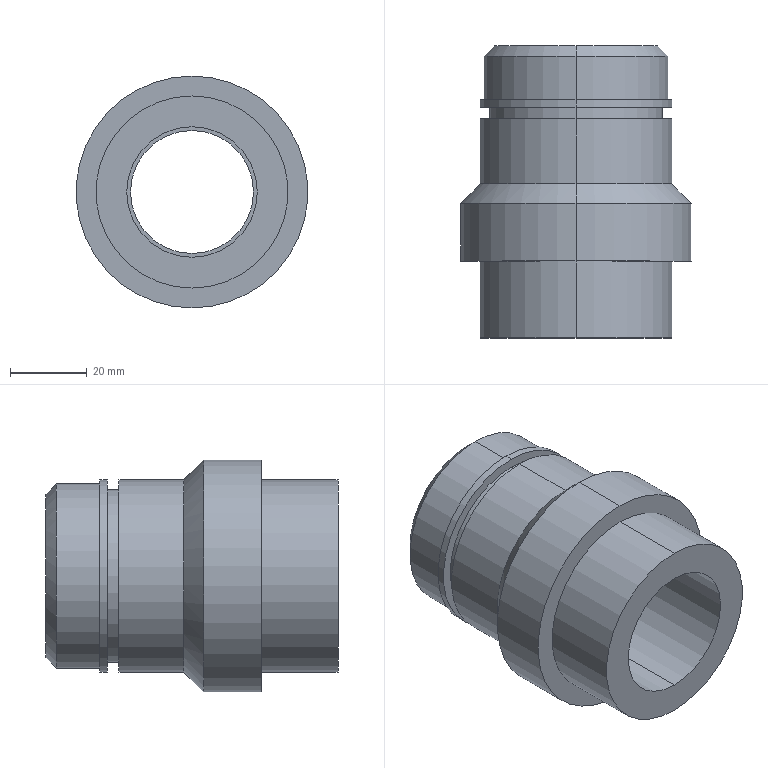Part | SolidWorks | features ICE 7, HoleWzd 2, Chamfer 1, Extrusion 1, StudWizard 1 | 1 solid | 27 faces | box 60.3 x 76 x 60.3 mm | volume 93894 mm3 | cylinder 16 | plane 7 | cone 4 | commonest cylinder face diameters 50 x6 32 x2 34 x2 45 x2 48 x2 60.3 x2
STEP:
#1=CARTESIAN_POINT('',(0.,58.,-16.));
#2=VERTEX_POINT('',#1);
#3=CARTESIAN_POINT('',(0.,58.,16.));
#4=VERTEX_POINT('',#3);
#5=CARTESIAN_POINT('',(0.,58.,0.));
#6=DIRECTION('',(0.,1.,0.));
#7=DIRECTION('',(0.,0.,1.));
#8=AXIS2_PLACEMENT_3D('',#5,#6,#7);
#9=CIRCLE('',#8,16.);
#10=EDGE_CURVE('',#2,#4,#9,.T.);
#11=ORIENTED_EDGE('',*,*,#10,.F.);
#12=CARTESIAN_POINT('',(0.,76.,-16.));
#13=VERTEX_POINT('',#12);
#14=CARTESIAN_POINT('',(0.,76.,-16.));
#15=DIRECTION('',(0.,1.,0.));
#16=VECTOR('',#15,1000.);
#17=LINE('',#14,#16);
#18=EDGE_CURVE('',#2,#13,#17,.T.);
#19=ORIENTED_EDGE('',*,*,#18,.T.);
#20=CARTESIAN_POINT('',(0.,76.,16.));
#21=VERTEX_POINT('',#20);
#22=CARTESIAN_POINT('',(0.,76.,0.));
#23=DIRECTION('',(0.,1.,0.));
#24=DIRECTION('',(0.,0.,1.));
#25=AXIS2_PLACEMENT_3D('',#22,#23,#24);
#26=CIRCLE('',#25,16.);
#27=EDGE_CURVE('',#13,#21,#26,.T.);
#28=ORIENTED_EDGE('',*,*,#27,.T.);
#29=CARTESIAN_POINT('',(0.,76.,16.));
#30=DIRECTION('',(0.,1.,0.));
#31=VECTOR('',#30,1000.);
#32=LINE('',#29,#31);
#33=EDGE_CURVE('',#4,#21,#32,.T.);
#34=ORIENTED_EDGE('',*,*,#33,.F.);
#35=EDGE_LOOP('',(#11,#19,#28,#34));
#36=FACE_OUTER_BOUND('',#35,.T.);
#37=CARTESIAN_POINT('',(0.,76.,0.));
#38=DIRECTION('',(0.,1.,0.));
#39=DIRECTION('',(0.,0.,1.));
#40=AXIS2_PLACEMENT_3D('',#37,#38,#39);
#41=CYLINDRICAL_SURFACE('',#40,16.);
#42=ADVANCED_FACE('',(#36),#41,.F.);
#43=CARTESIAN_POINT('',(0.,58.,17.));
#44=VERTEX_POINT('',#43);
#45=CARTESIAN_POINT('',(0.,58.,-17.));
#46=VERTEX_POINT('',#45);
#47=CARTESIAN_POINT('',(0.,58.,0.));
#48=DIRECTION('',(0.,-1.,0.));
#49=DIRECTION('',(0.,0.,1.));
#50=AXIS2_PLACEMENT_3D('',#47,#48,#49);
#51=CIRCLE('',#50,17.);
#52=EDGE_CURVE('',#44,#46,#51,.T.);
#53=ORIENTED_EDGE('',*,*,#52,.F.);
#54=CARTESIAN_POINT('',(0.,0.,17.));
#55=VERTEX_POINT('',#54);
#56=CARTESIAN_POINT('',(0.,0.,17.));
#57=DIRECTION('',(0.,-1.,0.));
#58=VECTOR('',#57,1000.);
#59=LINE('',#56,#58);
#60=EDGE_CURVE('',#44,#55,#59,.T.);
#61=ORIENTED_EDGE('',*,*,#60,.T.);
#62=CARTESIAN_POINT('',(0.,0.,-17.));
#63=VERTEX_POINT('',#62);
#64=CARTESIAN_POINT('',(0.,0.,0.));
#65=DIRECTION('',(0.,-1.,0.));
#66=DIRECTION('',(0.,0.,-1.));
#67=AXIS2_PLACEMENT_3D('',#64,#65,#66);
#68=CIRCLE('',#67,17.);
#69=EDGE_CURVE('',#55,#63,#68,.T.);
#70=ORIENTED_EDGE('',*,*,#69,.T.);
#71=CARTESIAN_POINT('',(0.,0.,-17.));
#72=DIRECTION('',(0.,-1.,0.));
#73=VECTOR('',#72,1000.);
#74=LINE('',#71,#73);
#75=EDGE_CURVE('',#46,#63,#74,.T.);
#76=ORIENTED_EDGE('',*,*,#75,.F.);
#77=EDGE_LOOP('',(#53,#61,#70,#76));
#78=FACE_OUTER_BOUND('',#77,.T.);
#79=CARTESIAN_POINT('',(0.,0.,0.));
#80=DIRECTION('',(0.,-1.,0.));
#81=DIRECTION('',(0.,0.,-1.));
#82=AXIS2_PLACEMENT_3D('',#79,#80,#81);
#83=CYLINDRICAL_SURFACE('',#82,17.);
#84=ADVANCED_FACE('',(#78),#83,.F.);
#85=CARTESIAN_POINT('',(0.,40.15,25.));
#86=VERTEX_POINT('',#85);
#87=CARTESIAN_POINT('',(0.,40.15,-25.));
#88=VERTEX_POINT('',#87);
#89=CARTESIAN_POINT('',(0.,40.15,0.));
#90=DIRECTION('',(0.,1.,0.));
#91=DIRECTION('',(0.,0.,-1.));
#92=AXIS2_PLACEMENT_3D('',#89,#90,#91);
#93=CIRCLE('',#92,25.);
#94=EDGE_CURVE('',#86,#88,#93,.T.);
#95=ORIENTED_EDGE('',*,*,#94,.F.);
#96=CARTESIAN_POINT('',(0.,35.,30.15));
#97=VERTEX_POINT('',#96);
#98=CARTESIAN_POINT('',(0.,35.,30.15));
#99=DIRECTION('',(0.,-0.7071,0.7071));
#100=VECTOR('',#99,1000.);
#101=LINE('',#98,#100);
#102=EDGE_CURVE('',#86,#97,#101,.T.);
#103=ORIENTED_EDGE('',*,*,#102,.T.);
#104=CARTESIAN_POINT('',(0.,35.,-30.15));
#105=VERTEX_POINT('',#104);
#106=CARTESIAN_POINT('',(0.,35.,0.));
#107=DIRECTION('',(0.,-1.,0.));
#108=DIRECTION('',(0.,0.,-1.));
#109=AXIS2_PLACEMENT_3D('',#106,#107,#108);
#110=CIRCLE('',#109,30.15);
#111=EDGE_CURVE('',#105,#97,#110,.T.);
#112=ORIENTED_EDGE('',*,*,#111,.F.);
#113=CARTESIAN_POINT('',(0.,35.,-30.15));
#114=DIRECTION('',(0.,-0.7071,-0.7071));
#115=VECTOR('',#114,1000.);
#116=LINE('',#113,#115);
#117=EDGE_CURVE('',#88,#105,#116,.T.);
#118=ORIENTED_EDGE('',*,*,#117,.F.);
#119=EDGE_LOOP('',(#95,#103,#112,#118));
#120=FACE_OUTER_BOUND('',#119,.T.);
#121=CARTESIAN_POINT('',(0.,35.,0.));
#122=DIRECTION('',(0.,-1.,0.));
#123=DIRECTION('',(0.,0.,-1.));
#124=AXIS2_PLACEMENT_3D('',#121,#122,#123);
#125=CONICAL_SURFACE('',#124,30.15,0.7854);
#126=ADVANCED_FACE('',(#120),#125,.T.);
#127=CARTESIAN_POINT('',(0.,20.,-25.));
#128=VERTEX_POINT('',#127);
#129=CARTESIAN_POINT('',(0.,20.,25.));
#130=VERTEX_POINT('',#129);
#131=CARTESIAN_POINT('',(0.,20.,0.));
#132=DIRECTION('',(0.,-1.,0.));
#133=DIRECTION('',(0.,0.,-1.));
#134=AXIS2_PLACEMENT_3D('',#131,#132,#133);
#135=CIRCLE('',#134,25.);
#136=EDGE_CURVE('',#128,#130,#135,.T.);
#137=ORIENTED_EDGE('',*,*,#136,.T.);
#138=CARTESIAN_POINT('',(0.,0.,25.));
#139=VERTEX_POINT('',#138);
#140=CARTESIAN_POINT('',(0.,57.,25.));
#141=DIRECTION('',(0.,-1.,0.));
#142=VECTOR('',#141,1000.);
#143=LINE('',#140,#142);
#144=EDGE_CURVE('',#130,#139,#143,.T.);
#145=ORIENTED_EDGE('',*,*,#144,.T.);
#146=CARTESIAN_POINT('',(0.,0.,-25.));
#147=VERTEX_POINT('',#146);
#148=CARTESIAN_POINT('',(0.,0.,0.));
#149=DIRECTION('',(0.,1.,0.));
#150=DIRECTION('',(0.,0.,1.));
#151=AXIS2_PLACEMENT_3D('',#148,#149,#150);
#152=CIRCLE('',#151,25.);
#153=EDGE_CURVE('',#139,#147,#152,.T.);
#154=ORIENTED_EDGE('',*,*,#153,.T.);
#155=CARTESIAN_POINT('',(0.,57.,-25.));
#156=DIRECTION('',(0.,-1.,0.));
#157=VECTOR('',#156,1000.);
#158=LINE('',#155,#157);
#159=EDGE_CURVE('',#128,#147,#158,.T.);
#160=ORIENTED_EDGE('',*,*,#159,.F.);
#161=EDGE_LOOP('',(#137,#145,#154,#160));
#162=FACE_OUTER_BOUND('',#161,.T.);
#163=CARTESIAN_POINT('',(0.,57.,0.));
#164=DIRECTION('',(0.,-1.,0.));
#165=DIRECTION('',(0.,0.,-1.));
#166=AXIS2_PLACEMENT_3D('',#163,#164,#165);
#167=CYLINDRICAL_SURFACE('',#166,25.);
#168=ADVANCED_FACE('',(#162),#167,.T.);
#169=ORIENTED_EDGE('',*,*,#111,.T.);
#170=CARTESIAN_POINT('',(0.,20.,30.15));
#171=VERTEX_POINT('',#170);
#172=CARTESIAN_POINT('',(0.,35.,30.15));
#173=DIRECTION('',(0.,-1.,0.));
#174=VECTOR('',#173,1000.);
#175=LINE('',#172,#174);
#176=EDGE_CURVE('',#97,#171,#175,.T.);
#177=ORIENTED_EDGE('',*,*,#176,.T.);
#178=CARTESIAN_POINT('',(0.,20.,-30.15));
#179=VERTEX_POINT('',#178);
#180=CARTESIAN_POINT('',(0.,20.,0.));
#181=DIRECTION('',(0.,-1.,0.));
#182=DIRECTION('',(0.,0.,-1.));
#183=AXIS2_PLACEMENT_3D('',#180,#181,#182);
#184=CIRCLE('',#183,30.15);
#185=EDGE_CURVE('',#179,#171,#184,.T.);
#186=ORIENTED_EDGE('',*,*,#185,.F.);
#187=CARTESIAN_POINT('',(0.,35.,-30.15));
#188=DIRECTION('',(0.,-1.,0.));
#189=VECTOR('',#188,1000.);
#190=LINE('',#187,#189);
#191=EDGE_CURVE('',#105,#179,#190,.T.);
#192=ORIENTED_EDGE('',*,*,#191,.F.);
#193=EDGE_LOOP('',(#169,#177,#186,#192));
#194=FACE_OUTER_BOUND('',#193,.T.);
#195=CARTESIAN_POINT('',(0.,35.,0.));
#196=DIRECTION('',(0.,-1.,0.));
#197=DIRECTION('',(0.,0.,-1.));
#198=AXIS2_PLACEMENT_3D('',#195,#196,#197);
#199=CYLINDRICAL_SURFACE('',#198,30.15);
#200=ADVANCED_FACE('',(#194),#199,.T.);
#201=CARTESIAN_POINT('',(0.,76.,-21.294));
#202=VERTEX_POINT('',#201);
#203=CARTESIAN_POINT('',(0.,76.,21.294));
#204=VERTEX_POINT('',#203);
#205=CARTESIAN_POINT('',(0.,76.,0.));
#206=DIRECTION('',(0.,-1.,0.));
#207=DIRECTION('',(0.,0.,-1.));
#208=AXIS2_PLACEMENT_3D('',#205,#206,#207);
#209=CIRCLE('',#208,21.294);
#210=EDGE_CURVE('',#202,#204,#209,.T.);
#211=ORIENTED_EDGE('',*,*,#210,.T.);
#212=CARTESIAN_POINT('',(0.,73.294,24.));
#213=VERTEX_POINT('',#212);
#214=CARTESIAN_POINT('',(0.,76.,21.294));
#215=DIRECTION('',(0.,-0.7071,0.7071));
#216=VECTOR('',#215,1000.);
#217=LINE('',#214,#216);
#218=EDGE_CURVE('',#204,#213,#217,.T.);
#219=ORIENTED_EDGE('',*,*,#218,.T.);
#220=CARTESIAN_POINT('',(0.,73.294,-24.));
#221=VERTEX_POINT('',#220);
#222=CARTESIAN_POINT('',(0.,73.294,0.));
#223=DIRECTION('',(0.,-1.,0.));
#224=DIRECTION('',(0.,0.,-1.));
#225=AXIS2_PLACEMENT_3D('',#222,#223,#224);
#226=CIRCLE('',#225,24.);
#227=EDGE_CURVE('',#221,#213,#226,.T.);
#228=ORIENTED_EDGE('',*,*,#227,.F.);
#229=CARTESIAN_POINT('',(0.,76.,-21.294));
#230=DIRECTION('',(0.,-0.7071,-0.7071));
#231=VECTOR('',#230,1000.);
#232=LINE('',#229,#231);
#233=EDGE_CURVE('',#202,#221,#232,.T.);
#234=ORIENTED_EDGE('',*,*,#233,.F.);
#235=EDGE_LOOP('',(#211,#219,#228,#234));
#236=FACE_OUTER_BOUND('',#235,.T.);
#237=CARTESIAN_POINT('',(0.,76.,0.));
#238=DIRECTION('',(0.,-1.,0.));
#239=DIRECTION('',(0.,0.,-1.));
#240=AXIS2_PLACEMENT_3D('',#237,#238,#239);
#241=CONICAL_SURFACE('',#240,21.294,0.7854);
#242=ADVANCED_FACE('',(#236),#241,.T.);
#243=ORIENTED_EDGE('',*,*,#227,.T.);
#244=CARTESIAN_POINT('',(0.,62.,24.));
#245=VERTEX_POINT('',#244);
#246=CARTESIAN_POINT('',(0.,76.,24.));
#247=DIRECTION('',(0.,-1.,0.));
#248=VECTOR('',#247,1000.);
#249=LINE('',#246,#248);
#250=EDGE_CURVE('',#213,#245,#249,.T.);
#251=ORIENTED_EDGE('',*,*,#250,.T.);
#252=CARTESIAN_POINT('',(0.,62.,-24.));
#253=VERTEX_POINT('',#252);
#254=CARTESIAN_POINT('',(0.,62.,0.));
#255=DIRECTION('',(0.,-1.,0.));
#256=DIRECTION('',(0.,0.,-1.));
#257=AXIS2_PLACEMENT_3D('',#254,#255,#256);
#258=CIRCLE('',#257,24.);
#259=EDGE_CURVE('',#253,#245,#258,.T.);
#260=ORIENTED_EDGE('',*,*,#259,.F.);
#261=CARTESIAN_POINT('',(0.,76.,-24.));
#262=DIRECTION('',(0.,-1.,0.));
#263=VECTOR('',#262,1000.);
#264=LINE('',#261,#263);
#265=EDGE_CURVE('',#221,#253,#264,.T.);
#266=ORIENTED_EDGE('',*,*,#265,.F.);
#267=EDGE_LOOP('',(#243,#251,#260,#266));
#268=FACE_OUTER_BOUND('',#267,.T.);
#269=CARTESIAN_POINT('',(0.,76.,0.));
#270=DIRECTION('',(0.,-1.,0.));
#271=DIRECTION('',(0.,0.,-1.));
#272=AXIS2_PLACEMENT_3D('',#269,#270,#271);
#273=CYLINDRICAL_SURFACE('',#272,24.);
#274=ADVANCED_FACE('',(#268),#273,.T.);
#275=CARTESIAN_POINT('',(0.,62.,25.));
#276=VERTEX_POINT('',#275);
#277=CARTESIAN_POINT('',(0.,62.,-25.));
#278=VERTEX_POINT('',#277);
#279=CARTESIAN_POINT('',(0.,62.,0.));
#280=DIRECTION('',(0.,1.,0.));
#281=DIRECTION('',(0.,0.,1.));
#282=AXIS2_PLACEMENT_3D('',#279,#280,#281);
#283=CIRCLE('',#282,25.);
#284=EDGE_CURVE('',#276,#278,#283,.T.);
#285=ORIENTED_EDGE('',*,*,#284,.F.);
#286=CARTESIAN_POINT('',(0.,60.,25.));
#287=VERTEX_POINT('',#286);
#288=CARTESIAN_POINT('',(0.,62.,25.));
#289=DIRECTION('',(0.,-1.,0.));
#290=VECTOR('',#289,1000.);
#291=LINE('',#288,#290);
#292=EDGE_CURVE('',#276,#287,#291,.T.);
#293=ORIENTED_EDGE('',*,*,#292,.T.);
#294=CARTESIAN_POINT('',(0.,60.,-25.));
#295=VERTEX_POINT('',#294);
#296=CARTESIAN_POINT('',(0.,60.,0.));
#297=DIRECTION('',(0.,1.,0.));
#298=DIRECTION('',(0.,0.,1.));
#299=AXIS2_PLACEMENT_3D('',#296,#297,#298);
#300=CIRCLE('',#299,25.);
#301=EDGE_CURVE('',#287,#295,#300,.T.);
#302=ORIENTED_EDGE('',*,*,#301,.T.);
#303=CARTESIAN_POINT('',(0.,62.,-25.));
#304=DIRECTION('',(0.,-1.,0.));
#305=VECTOR('',#304,1000.);
#306=LINE('',#303,#305);
#307=EDGE_CURVE('',#278,#295,#306,.T.);
#308=ORIENTED_EDGE('',*,*,#307,.F.);
#309=EDGE_LOOP('',(#285,#293,#302,#308));
#310=FACE_OUTER_BOUND('',#309,.T.);
#311=CARTESIAN_POINT('',(0.,62.,0.));
#312=DIRECTION('',(0.,-1.,0.));
#313=DIRECTION('',(0.,0.,-1.));
#314=AXIS2_PLACEMENT_3D('',#311,#312,#313);
#315=CYLINDRICAL_SURFACE('',#314,25.);
#316=ADVANCED_FACE('',(#310),#315,.T.);
#317=CARTESIAN_POINT('',(0.,60.,22.5));
#318=VERTEX_POINT('',#317);
#319=CARTESIAN_POINT('',(0.,60.,-22.5));
#320=VERTEX_POINT('',#319);
#321=CARTESIAN_POINT('',(0.,60.,0.));
#322=DIRECTION('',(0.,1.,0.));
#323=DIRECTION('',(0.,0.,1.));
#324=AXIS2_PLACEMENT_3D('',#321,#322,#323);
#325=CIRCLE('',#324,22.5);
#326=EDGE_CURVE('',#318,#320,#325,.T.);
#327=ORIENTED_EDGE('',*,*,#326,.F.);
#328=CARTESIAN_POINT('',(0.,57.,22.5));
#329=VERTEX_POINT('',#328);
#330=CARTESIAN_POINT('',(0.,60.,22.5));
#331=DIRECTION('',(0.,-1.,0.));
#332=VECTOR('',#331,1000.);
#333=LINE('',#330,#332);
#334=EDGE_CURVE('',#318,#329,#333,.T.);
#335=ORIENTED_EDGE('',*,*,#334,.T.);
#336=CARTESIAN_POINT('',(0.,57.,-22.5));
#337=VERTEX_POINT('',#336);
#338=CARTESIAN_POINT('',(0.,57.,0.));
#339=DIRECTION('',(0.,1.,0.));
#340=DIRECTION('',(0.,0.,1.));
#341=AXIS2_PLACEMENT_3D('',#338,#339,#340);
#342=CIRCLE('',#341,22.5);
#343=EDGE_CURVE('',#329,#337,#342,.T.);
#344=ORIENTED_EDGE('',*,*,#343,.T.);
#345=CARTESIAN_POINT('',(0.,60.,-22.5));
#346=DIRECTION('',(0.,-1.,0.));
#347=VECTOR('',#346,1000.);
#348=LINE('',#345,#347);
#349=EDGE_CURVE('',#320,#337,#348,.T.);
#350=ORIENTED_EDGE('',*,*,#349,.F.);
#351=EDGE_LOOP('',(#327,#335,#344,#350));
#352=FACE_OUTER_BOUND('',#351,.T.);
#353=CARTESIAN_POINT('',(0.,60.,0.));
#354=DIRECTION('',(0.,-1.,0.));
#355=DIRECTION('',(0.,0.,-1.));
#356=AXIS2_PLACEMENT_3D('',#353,#354,#355);
#357=CYLINDRICAL_SURFACE('',#356,22.5);
#358=ADVANCED_FACE('',(#352),#357,.T.);
#359=CARTESIAN_POINT('',(0.,57.,25.));
#360=VERTEX_POINT('',#359);
#361=CARTESIAN_POINT('',(0.,57.,-25.));
#362=VERTEX_POINT('',#361);
#363=CARTESIAN_POINT('',(0.,57.,0.));
#364=DIRECTION('',(0.,1.,0.));
#365=DIRECTION('',(0.,0.,1.));
#366=AXIS2_PLACEMENT_3D('',#363,#364,#365);
#367=CIRCLE('',#366,25.);
#368=EDGE_CURVE('',#360,#362,#367,.T.);
#369=ORIENTED_EDGE('',*,*,#368,.F.);
#370=CARTESIAN_POINT('',(0.,57.,25.));
#371=DIRECTION('',(0.,-1.,0.));
#372=VECTOR('',#371,1000.);
#373=LINE('',#370,#372);
#374=EDGE_CURVE('',#360,#86,#373,.T.);
#375=ORIENTED_EDGE('',*,*,#374,.T.);
#376=ORIENTED_EDGE('',*,*,#94,.T.);
#377=CARTESIAN_POINT('',(0.,57.,-25.));
#378=DIRECTION('',(0.,-1.,0.));
#379=VECTOR('',#378,1000.);
#380=LINE('',#377,#379);
#381=EDGE_CURVE('',#362,#88,#380,.T.);
#382=ORIENTED_EDGE('',*,*,#381,.F.);
#383=EDGE_LOOP('',(#369,#375,#376,#382));
#384=FACE_OUTER_BOUND('',#383,.T.);
#385=CARTESIAN_POINT('',(0.,57.,0.));
#386=DIRECTION('',(0.,-1.,0.));
#387=DIRECTION('',(0.,0.,-1.));
#388=AXIS2_PLACEMENT_3D('',#385,#386,#387);
#389=CYLINDRICAL_SURFACE('',#388,25.);
#390=ADVANCED_FACE('',(#384),#389,.T.);
#391=CARTESIAN_POINT('',(0.,0.,0.));
#392=DIRECTION('',(0.,1.,0.));
#393=DIRECTION('',(0.,0.,1.));
#394=AXIS2_PLACEMENT_3D('',#391,#392,#393);
#395=CIRCLE('',#394,25.);
#396=EDGE_CURVE('',#147,#139,#395,.T.);
#397=ORIENTED_EDGE('',*,*,#396,.F.);
#398=ORIENTED_EDGE('',*,*,#153,.F.);
#399=EDGE_LOOP('',(#397,#398));
#400=FACE_OUTER_BOUND('',#399,.T.);
#401=CARTESIAN_POINT('',(0.,0.,0.));
#402=DIRECTION('',(0.,-1.,0.));
#403=DIRECTION('',(0.,0.,-1.));
#404=AXIS2_PLACEMENT_3D('',#401,#402,#403);
#405=CIRCLE('',#404,17.);
#406=EDGE_CURVE('',#63,#55,#405,.T.);
#407=ORIENTED_EDGE('',*,*,#406,.F.);
#408=ORIENTED_EDGE('',*,*,#69,.F.);
#409=EDGE_LOOP('',(#407,#408));
#410=FACE_BOUND('',#409,.T.);
#411=CARTESIAN_POINT('',(0.,0.,0.));
#412=DIRECTION('',(0.,1.,0.));
#413=DIRECTION('',(0.,0.,1.));
#414=AXIS2_PLACEMENT_3D('',#411,#412,#413);
#415=PLANE('',#414);
#416=ADVANCED_FACE('',(#400,#410),#415,.F.);
#417=ORIENTED_EDGE('',*,*,#374,.F.);
#418=CARTESIAN_POINT('',(0.,57.,0.));
#419=DIRECTION('',(0.,1.,0.));
#420=DIRECTION('',(0.,0.,1.));
#421=AXIS2_PLACEMENT_3D('',#418,#419,#420);
#422=CIRCLE('',#421,25.);
#423=EDGE_CURVE('',#362,#360,#422,.T.);
#424=ORIENTED_EDGE('',*,*,#423,.F.);
#425=ORIENTED_EDGE('',*,*,#381,.T.);
#426=CARTESIAN_POINT('',(0.,40.15,0.));
#427=DIRECTION('',(0.,1.,0.));
#428=DIRECTION('',(0.,0.,-1.));
#429=AXIS2_PLACEMENT_3D('',#426,#427,#428);
#430=CIRCLE('',#429,25.);
#431=EDGE_CURVE('',#88,#86,#430,.T.);
#432=ORIENTED_EDGE('',*,*,#431,.T.);
#433=EDGE_LOOP('',(#417,#424,#425,#432));
#434=FACE_OUTER_BOUND('',#433,.T.);
#435=CARTESIAN_POINT('',(0.,57.,0.));
#436=DIRECTION('',(0.,-1.,0.));
#437=DIRECTION('',(0.,0.,-1.));
#438=AXIS2_PLACEMENT_3D('',#435,#436,#437);
#439=CYLINDRICAL_SURFACE('',#438,25.);
#440=ADVANCED_FACE('',(#434),#439,.T.);
#441=CARTESIAN_POINT('',(0.,57.,0.));
#442=DIRECTION('',(0.,1.,0.));
#443=DIRECTION('',(0.,0.,1.));
#444=AXIS2_PLACEMENT_3D('',#441,#442,#443);
#445=CIRCLE('',#444,22.5);
#446=EDGE_CURVE('',#337,#329,#445,.T.);
#447=ORIENTED_EDGE('',*,*,#446,.F.);
#448=ORIENTED_EDGE('',*,*,#343,.F.);
#449=EDGE_LOOP('',(#447,#448));
#450=FACE_BOUND('',#449,.T.);
#451=ORIENTED_EDGE('',*,*,#423,.T.);
#452=ORIENTED_EDGE('',*,*,#368,.T.);
#453=EDGE_LOOP('',(#451,#452));
#454=FACE_OUTER_BOUND('',#453,.T.);
#455=CARTESIAN_POINT('',(0.,57.,0.));
#456=DIRECTION('',(0.,1.,0.));
#457=DIRECTION('',(0.,0.,1.));
#458=AXIS2_PLACEMENT_3D('',#455,#456,#457);
#459=PLANE('',#458);
#460=ADVANCED_FACE('',(#450,#454),#459,.T.);
#461=ORIENTED_EDGE('',*,*,#334,.F.);
#462=CARTESIAN_POINT('',(0.,60.,0.));
#463=DIRECTION('',(0.,1.,0.));
#464=DIRECTION('',(0.,0.,1.));
#465=AXIS2_PLACEMENT_3D('',#462,#463,#464);
#466=CIRCLE('',#465,22.5);
#467=EDGE_CURVE('',#320,#318,#466,.T.);
#468=ORIENTED_EDGE('',*,*,#467,.F.);
#469=ORIENTED_EDGE('',*,*,#349,.T.);
#470=ORIENTED_EDGE('',*,*,#446,.T.);
#471=EDGE_LOOP('',(#461,#468,#469,#470));
#472=FACE_OUTER_BOUND('',#471,.T.);
#473=CARTESIAN_POINT('',(0.,60.,0.));
#474=DIRECTION('',(0.,-1.,0.));
#475=DIRECTION('',(0.,0.,-1.));
#476=AXIS2_PLACEMENT_3D('',#473,#474,#475);
#477=CYLINDRICAL_SURFACE('',#476,22.5);
#478=ADVANCED_FACE('',(#472),#477,.T.);
#479=ORIENTED_EDGE('',*,*,#292,.F.);
#480=CARTESIAN_POINT('',(0.,62.,0.));
#481=DIRECTION('',(0.,1.,0.));
#482=DIRECTION('',(0.,0.,1.));
#483=AXIS2_PLACEMENT_3D('',#480,#481,#482);
#484=CIRCLE('',#483,25.);
#485=EDGE_CURVE('',#278,#276,#484,.T.);
#486=ORIENTED_EDGE('',*,*,#485,.F.);
#487=ORIENTED_EDGE('',*,*,#307,.T.);
#488=CARTESIAN_POINT('',(0.,60.,0.));
#489=DIRECTION('',(0.,1.,0.));
#490=DIRECTION('',(0.,0.,1.));
#491=AXIS2_PLACEMENT_3D('',#488,#489,#490);
#492=CIRCLE('',#491,25.);
#493=EDGE_CURVE('',#295,#287,#492,.T.);
#494=ORIENTED_EDGE('',*,*,#493,.T.);
#495=EDGE_LOOP('',(#479,#486,#487,#494));
#496=FACE_OUTER_BOUND('',#495,.T.);
#497=CARTESIAN_POINT('',(0.,62.,0.));
#498=DIRECTION('',(0.,-1.,0.));
#499=DIRECTION('',(0.,0.,-1.));
#500=AXIS2_PLACEMENT_3D('',#497,#498,#499);
#501=CYLINDRICAL_SURFACE('',#500,25.);
#502=ADVANCED_FACE('',(#496),#501,.T.);
#503=ORIENTED_EDGE('',*,*,#485,.T.);
#504=ORIENTED_EDGE('',*,*,#284,.T.);
#505=EDGE_LOOP('',(#503,#504));
#506=FACE_OUTER_BOUND('',#505,.T.);
#507=ORIENTED_EDGE('',*,*,#259,.T.);
#508=CARTESIAN_POINT('',(0.,62.,0.));
#509=DIRECTION('',(0.,-1.,0.));
#510=DIRECTION('',(0.,0.,-1.));
#511=AXIS2_PLACEMENT_3D('',#508,#509,#510);
#512=CIRCLE('',#511,24.);
#513=EDGE_CURVE('',#245,#253,#512,.T.);
#514=ORIENTED_EDGE('',*,*,#513,.T.);
#515=EDGE_LOOP('',(#507,#514));
#516=FACE_BOUND('',#515,.T.);
#517=CARTESIAN_POINT('',(0.,62.,0.));
#518=DIRECTION('',(0.,1.,0.));
#519=DIRECTION('',(0.,0.,1.));
#520=AXIS2_PLACEMENT_3D('',#517,#518,#519);
#521=PLANE('',#520);
#522=ADVANCED_FACE('',(#506,#516),#521,.T.);
#523=ORIENTED_EDGE('',*,*,#467,.T.);
#524=ORIENTED_EDGE('',*,*,#326,.T.);
#525=EDGE_LOOP('',(#523,#524));
#526=FACE_BOUND('',#525,.T.);
#527=ORIENTED_EDGE('',*,*,#493,.F.);
#528=ORIENTED_EDGE('',*,*,#301,.F.);
#529=EDGE_LOOP('',(#527,#528));
#530=FACE_OUTER_BOUND('',#529,.T.);
#531=CARTESIAN_POINT('',(0.,60.,0.));
#532=DIRECTION('',(0.,1.,0.));
#533=DIRECTION('',(0.,0.,1.));
#534=AXIS2_PLACEMENT_3D('',#531,#532,#533);
#535=PLANE('',#534);
#536=ADVANCED_FACE('',(#526,#530),#535,.F.);
#537=ORIENTED_EDGE('',*,*,#250,.F.);
#538=CARTESIAN_POINT('',(0.,73.294,0.));
#539=DIRECTION('',(0.,-1.,0.));
#540=DIRECTION('',(0.,0.,-1.));
#541=AXIS2_PLACEMENT_3D('',#538,#539,#540);
#542=CIRCLE('',#541,24.);
#543=EDGE_CURVE('',#213,#221,#542,.T.);
#544=ORIENTED_EDGE('',*,*,#543,.T.);
#545=ORIENTED_EDGE('',*,*,#265,.T.);
#546=ORIENTED_EDGE('',*,*,#513,.F.);
#547=EDGE_LOOP('',(#537,#544,#545,#546));
#548=FACE_OUTER_BOUND('',#547,.T.);
#549=CARTESIAN_POINT('',(0.,76.,0.));
#550=DIRECTION('',(0.,-1.,0.));
#551=DIRECTION('',(0.,0.,-1.));
#552=AXIS2_PLACEMENT_3D('',#549,#550,#551);
#553=CYLINDRICAL_SURFACE('',#552,24.);
#554=ADVANCED_FACE('',(#548),#553,.T.);
#555=ORIENTED_EDGE('',*,*,#218,.F.);
#556=CARTESIAN_POINT('',(0.,76.,0.));
#557=DIRECTION('',(0.,-1.,0.));
#558=DIRECTION('',(0.,0.,-1.));
#559=AXIS2_PLACEMENT_3D('',#556,#557,#558);
#560=CIRCLE('',#559,21.294);
#561=EDGE_CURVE('',#204,#202,#560,.T.);
#562=ORIENTED_EDGE('',*,*,#561,.T.);
#563=ORIENTED_EDGE('',*,*,#233,.T.);
#564=ORIENTED_EDGE('',*,*,#543,.F.);
#565=EDGE_LOOP('',(#555,#562,#563,#564));
#566=FACE_OUTER_BOUND('',#565,.T.);
#567=CARTESIAN_POINT('',(0.,76.,0.));
#568=DIRECTION('',(0.,-1.,0.));
#569=DIRECTION('',(0.,0.,-1.));
#570=AXIS2_PLACEMENT_3D('',#567,#568,#569);
#571=CONICAL_SURFACE('',#570,21.294,0.7854);
#572=ADVANCED_FACE('',(#566),#571,.T.);
#573=CARTESIAN_POINT('',(0.,76.,0.));
#574=DIRECTION('',(0.,1.,0.));
#575=DIRECTION('',(0.,0.,1.));
#576=AXIS2_PLACEMENT_3D('',#573,#574,#575);
#577=CIRCLE('',#576,16.);
#578=EDGE_CURVE('',#21,#13,#577,.T.);
#579=ORIENTED_EDGE('',*,*,#578,.F.);
#580=ORIENTED_EDGE('',*,*,#27,.F.);
#581=EDGE_LOOP('',(#579,#580));
#582=FACE_BOUND('',#581,.T.);
#583=ORIENTED_EDGE('',*,*,#210,.F.);
#584=ORIENTED_EDGE('',*,*,#561,.F.);
#585=EDGE_LOOP('',(#583,#584));
#586=FACE_OUTER_BOUND('',#585,.T.);
#587=CARTESIAN_POINT('',(0.,76.,0.));
#588=DIRECTION('',(0.,1.,0.));
#589=DIRECTION('',(0.,0.,1.));
#590=AXIS2_PLACEMENT_3D('',#587,#588,#589);
#591=PLANE('',#590);
#592=ADVANCED_FACE('',(#582,#586),#591,.T.);
#593=ORIENTED_EDGE('',*,*,#176,.F.);
#594=CARTESIAN_POINT('',(0.,35.,0.));
#595=DIRECTION('',(0.,-1.,0.));
#596=DIRECTION('',(0.,0.,-1.));
#597=AXIS2_PLACEMENT_3D('',#594,#595,#596);
#598=CIRCLE('',#597,30.15);
#599=EDGE_CURVE('',#97,#105,#598,.T.);
#600=ORIENTED_EDGE('',*,*,#599,.T.);
#601=ORIENTED_EDGE('',*,*,#191,.T.);
#602=CARTESIAN_POINT('',(0.,20.,0.));
#603=DIRECTION('',(0.,-1.,0.));
#604=DIRECTION('',(0.,0.,-1.));
#605=AXIS2_PLACEMENT_3D('',#602,#603,#604);
#606=CIRCLE('',#605,30.15);
#607=EDGE_CURVE('',#171,#179,#606,.T.);
#608=ORIENTED_EDGE('',*,*,#607,.F.);
#609=EDGE_LOOP('',(#593,#600,#601,#608));
#610=FACE_OUTER_BOUND('',#609,.T.);
#611=CARTESIAN_POINT('',(0.,35.,0.));
#612=DIRECTION('',(0.,-1.,0.));
#613=DIRECTION('',(0.,0.,-1.));
#614=AXIS2_PLACEMENT_3D('',#611,#612,#613);
#615=CYLINDRICAL_SURFACE('',#614,30.15);
#616=ADVANCED_FACE('',(#610),#615,.T.);
#617=ORIENTED_EDGE('',*,*,#136,.F.);
#618=CARTESIAN_POINT('',(0.,20.,0.));
#619=DIRECTION('',(0.,-1.,0.));
#620=DIRECTION('',(0.,0.,-1.));
#621=AXIS2_PLACEMENT_3D('',#618,#619,#620);
#622=CIRCLE('',#621,25.);
#623=EDGE_CURVE('',#130,#128,#622,.T.);
#624=ORIENTED_EDGE('',*,*,#623,.F.);
#625=EDGE_LOOP('',(#617,#624));
#626=FACE_BOUND('',#625,.T.);
#627=ORIENTED_EDGE('',*,*,#185,.T.);
#628=ORIENTED_EDGE('',*,*,#607,.T.);
#629=EDGE_LOOP('',(#627,#628));
#630=FACE_OUTER_BOUND('',#629,.T.);
#631=CARTESIAN_POINT('',(0.,20.,0.));
#632=DIRECTION('',(0.,-1.,0.));
#633=DIRECTION('',(0.,0.,-1.));
#634=AXIS2_PLACEMENT_3D('',#631,#632,#633);
#635=PLANE('',#634);
#636=ADVANCED_FACE('',(#626,#630),#635,.T.);
#637=ORIENTED_EDGE('',*,*,#144,.F.);
#638=ORIENTED_EDGE('',*,*,#623,.T.);
#639=ORIENTED_EDGE('',*,*,#159,.T.);
#640=ORIENTED_EDGE('',*,*,#396,.T.);
#641=EDGE_LOOP('',(#637,#638,#639,#640));
#642=FACE_OUTER_BOUND('',#641,.T.);
#643=CARTESIAN_POINT('',(0.,57.,0.));
#644=DIRECTION('',(0.,-1.,0.));
#645=DIRECTION('',(0.,0.,-1.));
#646=AXIS2_PLACEMENT_3D('',#643,#644,#645);
#647=CYLINDRICAL_SURFACE('',#646,25.);
#648=ADVANCED_FACE('',(#642),#647,.T.);
#649=ORIENTED_EDGE('',*,*,#102,.F.);
#650=ORIENTED_EDGE('',*,*,#431,.F.);
#651=ORIENTED_EDGE('',*,*,#117,.T.);
#652=ORIENTED_EDGE('',*,*,#599,.F.);
#653=EDGE_LOOP('',(#649,#650,#651,#652));
#654=FACE_OUTER_BOUND('',#653,.T.);
#655=CARTESIAN_POINT('',(0.,35.,0.));
#656=DIRECTION('',(0.,-1.,0.));
#657=DIRECTION('',(0.,0.,-1.));
#658=AXIS2_PLACEMENT_3D('',#655,#656,#657);
#659=CONICAL_SURFACE('',#658,30.15,0.7854);
#660=ADVANCED_FACE('',(#654),#659,.T.);
#661=ORIENTED_EDGE('',*,*,#60,.F.);
#662=CARTESIAN_POINT('',(0.,58.,0.));
#663=DIRECTION('',(0.,-1.,0.));
#664=DIRECTION('',(0.,0.,1.));
#665=AXIS2_PLACEMENT_3D('',#662,#663,#664);
#666=CIRCLE('',#665,17.);
#667=EDGE_CURVE('',#46,#44,#666,.T.);
#668=ORIENTED_EDGE('',*,*,#667,.F.);
#669=ORIENTED_EDGE('',*,*,#75,.T.);
#670=ORIENTED_EDGE('',*,*,#406,.T.);
#671=EDGE_LOOP('',(#661,#668,#669,#670));
#672=FACE_OUTER_BOUND('',#671,.T.);
#673=CARTESIAN_POINT('',(0.,0.,0.));
#674=DIRECTION('',(0.,-1.,0.));
#675=DIRECTION('',(0.,0.,-1.));
#676=AXIS2_PLACEMENT_3D('',#673,#674,#675);
#677=CYLINDRICAL_SURFACE('',#676,17.);
#678=ADVANCED_FACE('',(#672),#677,.F.);
#679=ORIENTED_EDGE('',*,*,#18,.F.);
#680=CARTESIAN_POINT('',(0.,58.,0.));
#681=DIRECTION('',(0.,1.,0.));
#682=DIRECTION('',(0.,0.,1.));
#683=AXIS2_PLACEMENT_3D('',#680,#681,#682);
#684=CIRCLE('',#683,16.);
#685=EDGE_CURVE('',#4,#2,#684,.T.);
#686=ORIENTED_EDGE('',*,*,#685,.F.);
#687=ORIENTED_EDGE('',*,*,#33,.T.);
#688=ORIENTED_EDGE('',*,*,#578,.T.);
#689=EDGE_LOOP('',(#679,#686,#687,#688));
#690=FACE_OUTER_BOUND('',#689,.T.);
#691=CARTESIAN_POINT('',(0.,76.,0.));
#692=DIRECTION('',(0.,1.,0.));
#693=DIRECTION('',(0.,0.,1.));
#694=AXIS2_PLACEMENT_3D('',#691,#692,#693);
#695=CYLINDRICAL_SURFACE('',#694,16.);
#696=ADVANCED_FACE('',(#690),#695,.F.);
#697=ORIENTED_EDGE('',*,*,#685,.T.);
#698=ORIENTED_EDGE('',*,*,#10,.T.);
#699=EDGE_LOOP('',(#697,#698));
#700=FACE_BOUND('',#699,.T.);
#701=ORIENTED_EDGE('',*,*,#667,.T.);
#702=ORIENTED_EDGE('',*,*,#52,.T.);
#703=EDGE_LOOP('',(#701,#702));
#704=FACE_OUTER_BOUND('',#703,.T.);
#705=CARTESIAN_POINT('',(0.,58.,0.));
#706=DIRECTION('',(0.,1.,0.));
#707=DIRECTION('',(0.,0.,1.));
#708=AXIS2_PLACEMENT_3D('',#705,#706,#707);
#709=PLANE('',#708);
#710=ADVANCED_FACE('',(#700,#704),#709,.F.);
#711=CLOSED_SHELL('',(#42,#84,#126,#168,#200,#242,#274,#316,#358,#390,#416,#440,#460,#478,#502,#522,#536,#554,#572,#592,#616,#636,#648,#660,#678,#696,#710));
#712=MANIFOLD_SOLID_BREP('',#711);
#713=CARTESIAN_POINT('',(0.,0.,0.));
#714=DIRECTION('',(0.,0.,1.));
#715=DIRECTION('',(1.,0.,0.));
#716=AXIS2_PLACEMENT_3D('',#713,#714,#715);
#717=(LENGTH_UNIT()NAMED_UNIT(*)SI_UNIT(.MILLI.,.METRE.));
#718=UNCERTAINTY_MEASURE_WITH_UNIT(LENGTH_MEASURE(0.00001),#717,'','');
#719=(NAMED_UNIT(*)PLANE_ANGLE_UNIT()SI_UNIT($,.RADIAN.));
#720=(NAMED_UNIT(*)SI_UNIT($,.STERADIAN.)SOLID_ANGLE_UNIT());
#721=(GEOMETRIC_REPRESENTATION_CONTEXT(3)GLOBAL_UNCERTAINTY_ASSIGNED_CONTEXT((#718))GLOBAL_UNIT_ASSIGNED_CONTEXT((#717,#719,#720))REPRESENTATION_CONTEXT('',''));
#722=ADVANCED_BREP_SHAPE_REPRESENTATION('',(#712,#716),#721);